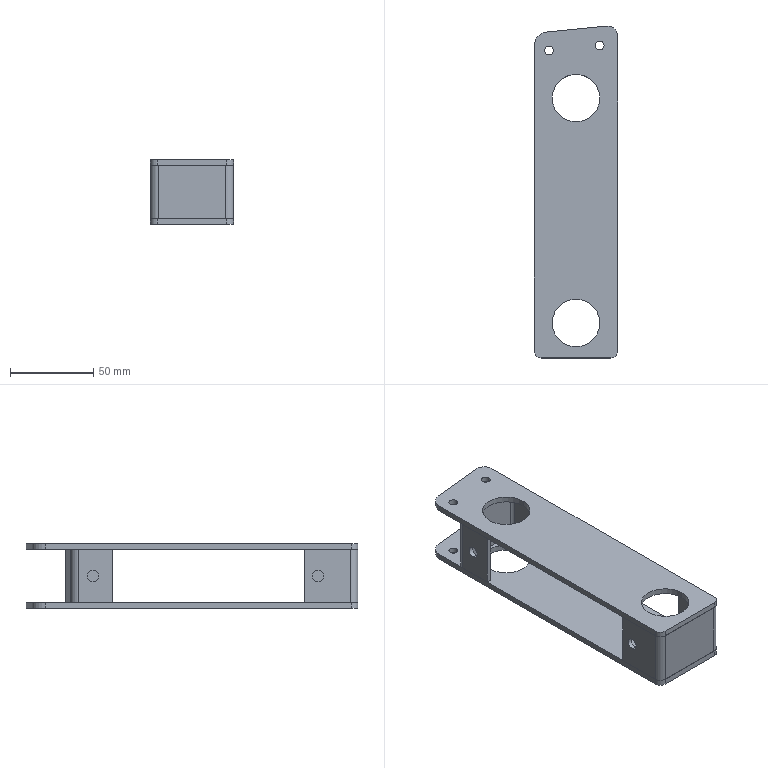Part | STEP file | BASE RIEL SUPERIOR_SLIM V2 | 4 solids | 84 faces | box 50 x 199.37 x 39 mm | volume 75917 mm3 | plane 48 | cylinder 36 | commonest cylinder face diameters 5.3 x8 28.6 x8 4 x4 6.8 x4 8 x4 9.2 x4